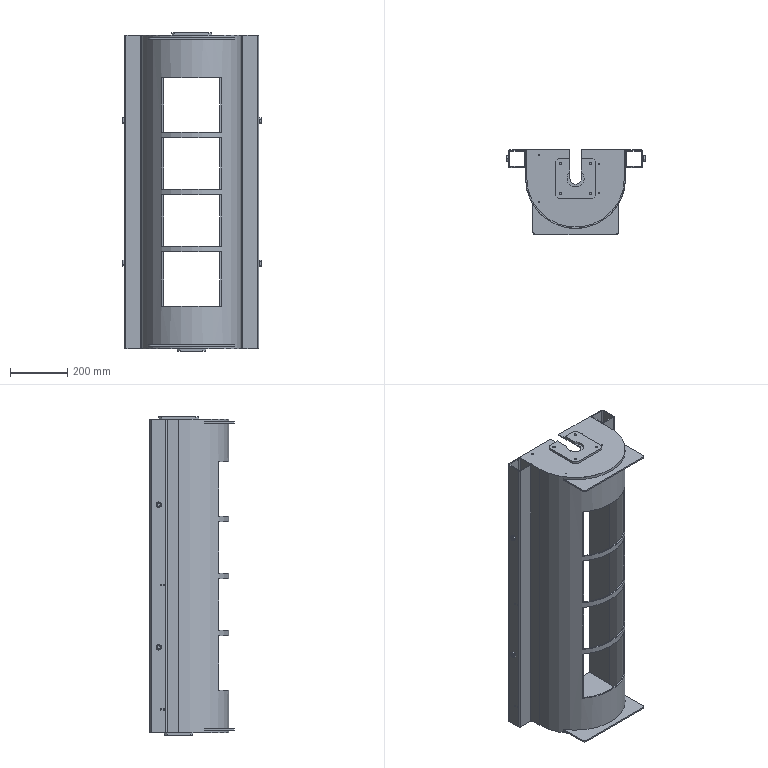Part | SolidWorks | features ICE 12, HoleWzd 7, Fillet 4, MoveCopyBody 4, Chamfer 3, LPattern 3, Stock 3, Cut 1, Extrusion 1, Shell 1 | 10 solids | 336 faces | box 487 x 297 x 1116 mm | volume 5128142 mm3 | cylinder 156 | plane 156 | cone 24 | commonest cylinder face diameters 4.2 x60 8.5 x24 10 x16 15 x16 10.376 x8 14.75 x8